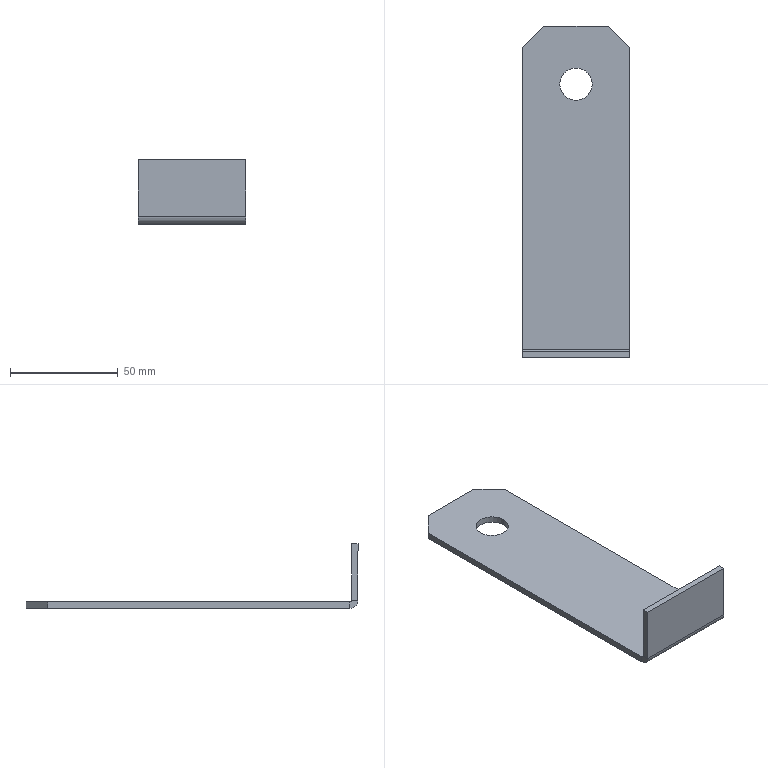Part | SolidWorks | features Chamfer 1, EdgeFlange 1, FlatPattern 1, ICE 1, SMBaseFlange 1, SheetMetal 1 | 1 solid | 18 faces | box 50 x 154 x 30 mm | volume 26176 mm3 | plane 14 | cylinder 4 | commonest cylinder face diameters 15 x2 1.473 x1 7.473 x1
STEP:
#1=CARTESIAN_POINT('',(7.5,50.,0.));
#2=VERTEX_POINT('',#1);
#3=CARTESIAN_POINT('',(-7.5,50.,0.));
#4=VERTEX_POINT('',#3);
#5=CARTESIAN_POINT('',(0.,50.,0.));
#6=DIRECTION('',(0.,0.,-1.));
#7=DIRECTION('',(-1.,0.,0.));
#8=AXIS2_PLACEMENT_3D('',#5,#6,#7);
#9=CIRCLE('',#8,7.5);
#10=EDGE_CURVE('',#2,#4,#9,.T.);
#11=ORIENTED_EDGE('',*,*,#10,.F.);
#12=CARTESIAN_POINT('',(7.5,50.,-3.));
#13=VERTEX_POINT('',#12);
#14=CARTESIAN_POINT('',(7.5,50.,27.));
#15=DIRECTION('',(0.,0.,-1.));
#16=VECTOR('',#15,1000.);
#17=LINE('',#14,#16);
#18=EDGE_CURVE('',#2,#13,#17,.T.);
#19=ORIENTED_EDGE('',*,*,#18,.T.);
#20=CARTESIAN_POINT('',(-7.5,50.,-3.));
#21=VERTEX_POINT('',#20);
#22=CARTESIAN_POINT('',(0.,50.,-3.));
#23=DIRECTION('',(0.,0.,-1.));
#24=DIRECTION('',(-1.,0.,0.));
#25=AXIS2_PLACEMENT_3D('',#22,#23,#24);
#26=CIRCLE('',#25,7.5);
#27=EDGE_CURVE('',#13,#21,#26,.T.);
#28=ORIENTED_EDGE('',*,*,#27,.T.);
#29=CARTESIAN_POINT('',(-7.5,50.,27.));
#30=DIRECTION('',(0.,0.,-1.));
#31=VECTOR('',#30,1000.);
#32=LINE('',#29,#31);
#33=EDGE_CURVE('',#4,#21,#32,.T.);
#34=ORIENTED_EDGE('',*,*,#33,.F.);
#35=EDGE_LOOP('',(#11,#19,#28,#34));
#36=FACE_OUTER_BOUND('',#35,.T.);
#37=CARTESIAN_POINT('',(0.,50.,27.));
#38=DIRECTION('',(0.,0.,-1.));
#39=DIRECTION('',(-1.,0.,0.));
#40=AXIS2_PLACEMENT_3D('',#37,#38,#39);
#41=CYLINDRICAL_SURFACE('',#40,7.5);
#42=ADVANCED_FACE('',(#36),#41,.F.);
#43=CARTESIAN_POINT('',(25.,-73.263,-3.));
#44=VERTEX_POINT('',#43);
#45=CARTESIAN_POINT('',(25.,67.,-3.));
#46=VERTEX_POINT('',#45);
#47=CARTESIAN_POINT('',(25.,-77.,-3.));
#48=DIRECTION('',(0.,1.,0.));
#49=VECTOR('',#48,1000.);
#50=LINE('',#47,#49);
#51=EDGE_CURVE('',#44,#46,#50,.T.);
#52=ORIENTED_EDGE('',*,*,#51,.T.);
#53=CARTESIAN_POINT('',(25.,67.,0.));
#54=VERTEX_POINT('',#53);
#55=CARTESIAN_POINT('',(25.,67.,-3.));
#56=DIRECTION('',(0.,0.,1.));
#57=VECTOR('',#56,1000.);
#58=LINE('',#55,#57);
#59=EDGE_CURVE('',#46,#54,#58,.T.);
#60=ORIENTED_EDGE('',*,*,#59,.T.);
#61=CARTESIAN_POINT('',(25.,-73.263,0.));
#62=VERTEX_POINT('',#61);
#63=CARTESIAN_POINT('',(25.,-77.,0.));
#64=DIRECTION('',(0.,1.,0.));
#65=VECTOR('',#64,1000.);
#66=LINE('',#63,#65);
#67=EDGE_CURVE('',#62,#54,#66,.T.);
#68=ORIENTED_EDGE('',*,*,#67,.F.);
#69=CARTESIAN_POINT('',(25.,-73.263,0.));
#70=DIRECTION('',(0.,0.,-1.));
#71=VECTOR('',#70,1000.);
#72=LINE('',#69,#71);
#73=EDGE_CURVE('',#62,#44,#72,.T.);
#74=ORIENTED_EDGE('',*,*,#73,.T.);
#75=EDGE_LOOP('',(#52,#60,#68,#74));
#76=FACE_OUTER_BOUND('',#75,.T.);
#77=CARTESIAN_POINT('',(25.,-77.,-3.));
#78=DIRECTION('',(1.,0.,0.));
#79=DIRECTION('',(0.,0.,-1.));
#80=AXIS2_PLACEMENT_3D('',#77,#78,#79);
#81=PLANE('',#80);
#82=ADVANCED_FACE('',(#76),#81,.T.);
#83=CARTESIAN_POINT('',(0.,50.,-3.));
#84=DIRECTION('',(0.,0.,-1.));
#85=DIRECTION('',(-1.,0.,0.));
#86=AXIS2_PLACEMENT_3D('',#83,#84,#85);
#87=CIRCLE('',#86,7.5);
#88=EDGE_CURVE('',#21,#13,#87,.T.);
#89=ORIENTED_EDGE('',*,*,#88,.F.);
#90=ORIENTED_EDGE('',*,*,#27,.F.);
#91=EDGE_LOOP('',(#89,#90));
#92=FACE_BOUND('',#91,.T.);
#93=CARTESIAN_POINT('',(-25.,67.,-3.));
#94=VERTEX_POINT('',#93);
#95=CARTESIAN_POINT('',(-25.,-73.263,-3.));
#96=VERTEX_POINT('',#95);
#97=CARTESIAN_POINT('',(-25.,-77.,-3.));
#98=DIRECTION('',(0.,-1.,0.));
#99=VECTOR('',#98,1000.);
#100=LINE('',#97,#99);
#101=EDGE_CURVE('',#94,#96,#100,.T.);
#102=ORIENTED_EDGE('',*,*,#101,.F.);
#103=CARTESIAN_POINT('',(-15.,77.,-3.));
#104=VERTEX_POINT('',#103);
#105=CARTESIAN_POINT('',(-46.,46.,-3.));
#106=DIRECTION('',(0.7071,0.7071,0.));
#107=VECTOR('',#106,1000.);
#108=LINE('',#105,#107);
#109=EDGE_CURVE('',#94,#104,#108,.T.);
#110=ORIENTED_EDGE('',*,*,#109,.T.);
#111=CARTESIAN_POINT('',(15.,77.,-3.));
#112=VERTEX_POINT('',#111);
#113=CARTESIAN_POINT('',(-25.,77.,-3.));
#114=DIRECTION('',(-1.,0.,0.));
#115=VECTOR('',#114,1000.);
#116=LINE('',#113,#115);
#117=EDGE_CURVE('',#112,#104,#116,.T.);
#118=ORIENTED_EDGE('',*,*,#117,.F.);
#119=CARTESIAN_POINT('',(46.,46.,-3.));
#120=DIRECTION('',(0.7071,-0.7071,0.));
#121=VECTOR('',#120,1000.);
#122=LINE('',#119,#121);
#123=EDGE_CURVE('',#112,#46,#122,.T.);
#124=ORIENTED_EDGE('',*,*,#123,.T.);
#125=ORIENTED_EDGE('',*,*,#51,.F.);
#126=CARTESIAN_POINT('',(25.,-73.263,-3.));
#127=DIRECTION('',(-1.,0.,0.));
#128=VECTOR('',#127,1000.);
#129=LINE('',#126,#128);
#130=EDGE_CURVE('',#44,#96,#129,.T.);
#131=ORIENTED_EDGE('',*,*,#130,.T.);
#132=EDGE_LOOP('',(#102,#110,#118,#124,#125,#131));
#133=FACE_OUTER_BOUND('',#132,.T.);
#134=CARTESIAN_POINT('',(0.,0.,-3.));
#135=DIRECTION('',(0.,0.,-1.));
#136=DIRECTION('',(-1.,0.,0.));
#137=AXIS2_PLACEMENT_3D('',#134,#135,#136);
#138=PLANE('',#137);
#139=ADVANCED_FACE('',(#92,#133),#138,.T.);
#140=CARTESIAN_POINT('',(0.,50.,0.));
#141=DIRECTION('',(0.,0.,-1.));
#142=DIRECTION('',(-1.,0.,0.));
#143=AXIS2_PLACEMENT_3D('',#140,#141,#142);
#144=CIRCLE('',#143,7.5);
#145=EDGE_CURVE('',#4,#2,#144,.T.);
#146=ORIENTED_EDGE('',*,*,#145,.T.);
#147=ORIENTED_EDGE('',*,*,#10,.T.);
#148=EDGE_LOOP('',(#146,#147));
#149=FACE_BOUND('',#148,.T.);
#150=CARTESIAN_POINT('',(15.,77.,0.));
#151=VERTEX_POINT('',#150);
#152=CARTESIAN_POINT('',(-15.,77.,0.));
#153=VERTEX_POINT('',#152);
#154=CARTESIAN_POINT('',(-25.,77.,0.));
#155=DIRECTION('',(-1.,0.,0.));
#156=VECTOR('',#155,1000.);
#157=LINE('',#154,#156);
#158=EDGE_CURVE('',#151,#153,#157,.T.);
#159=ORIENTED_EDGE('',*,*,#158,.T.);
#160=CARTESIAN_POINT('',(-25.,67.,0.));
#161=VERTEX_POINT('',#160);
#162=CARTESIAN_POINT('',(-15.,77.,0.));
#163=DIRECTION('',(-0.7071,-0.7071,0.));
#164=VECTOR('',#163,1000.);
#165=LINE('',#162,#164);
#166=EDGE_CURVE('',#153,#161,#165,.T.);
#167=ORIENTED_EDGE('',*,*,#166,.T.);
#168=CARTESIAN_POINT('',(-25.,-73.263,0.));
#169=VERTEX_POINT('',#168);
#170=CARTESIAN_POINT('',(-25.,-77.,0.));
#171=DIRECTION('',(0.,-1.,0.));
#172=VECTOR('',#171,1000.);
#173=LINE('',#170,#172);
#174=EDGE_CURVE('',#161,#169,#173,.T.);
#175=ORIENTED_EDGE('',*,*,#174,.T.);
#176=CARTESIAN_POINT('',(25.,-73.263,0.));
#177=DIRECTION('',(-1.,0.,0.));
#178=VECTOR('',#177,1000.);
#179=LINE('',#176,#178);
#180=EDGE_CURVE('',#62,#169,#179,.T.);
#181=ORIENTED_EDGE('',*,*,#180,.F.);
#182=ORIENTED_EDGE('',*,*,#67,.T.);
#183=CARTESIAN_POINT('',(25.,67.,0.));
#184=DIRECTION('',(-0.7071,0.7071,0.));
#185=VECTOR('',#184,1000.);
#186=LINE('',#183,#185);
#187=EDGE_CURVE('',#54,#151,#186,.T.);
#188=ORIENTED_EDGE('',*,*,#187,.T.);
#189=EDGE_LOOP('',(#159,#167,#175,#181,#182,#188));
#190=FACE_OUTER_BOUND('',#189,.T.);
#191=CARTESIAN_POINT('',(0.,0.,0.));
#192=DIRECTION('',(0.,0.,-1.));
#193=DIRECTION('',(-1.,0.,0.));
#194=AXIS2_PLACEMENT_3D('',#191,#192,#193);
#195=PLANE('',#194);
#196=ADVANCED_FACE('',(#149,#190),#195,.F.);
#197=ORIENTED_EDGE('',*,*,#174,.F.);
#198=CARTESIAN_POINT('',(-25.,67.,-3.));
#199=DIRECTION('',(0.,0.,-1.));
#200=VECTOR('',#199,1000.);
#201=LINE('',#198,#200);
#202=EDGE_CURVE('',#161,#94,#201,.T.);
#203=ORIENTED_EDGE('',*,*,#202,.T.);
#204=ORIENTED_EDGE('',*,*,#101,.T.);
#205=CARTESIAN_POINT('',(-25.,-73.263,0.));
#206=DIRECTION('',(0.,0.,-1.));
#207=VECTOR('',#206,1000.);
#208=LINE('',#205,#207);
#209=EDGE_CURVE('',#169,#96,#208,.T.);
#210=ORIENTED_EDGE('',*,*,#209,.F.);
#211=EDGE_LOOP('',(#197,#203,#204,#210));
#212=FACE_OUTER_BOUND('',#211,.T.);
#213=CARTESIAN_POINT('',(-25.,-77.,-3.));
#214=DIRECTION('',(-1.,0.,0.));
#215=DIRECTION('',(0.,0.,1.));
#216=AXIS2_PLACEMENT_3D('',#213,#214,#215);
#217=PLANE('',#216);
#218=ADVANCED_FACE('',(#212),#217,.T.);
#219=ORIENTED_EDGE('',*,*,#117,.T.);
#220=CARTESIAN_POINT('',(-15.,77.,-3.));
#221=DIRECTION('',(0.,0.,1.));
#222=VECTOR('',#221,1000.);
#223=LINE('',#220,#222);
#224=EDGE_CURVE('',#104,#153,#223,.T.);
#225=ORIENTED_EDGE('',*,*,#224,.T.);
#226=ORIENTED_EDGE('',*,*,#158,.F.);
#227=CARTESIAN_POINT('',(15.,77.,-3.));
#228=DIRECTION('',(0.,0.,-1.));
#229=VECTOR('',#228,1000.);
#230=LINE('',#227,#229);
#231=EDGE_CURVE('',#151,#112,#230,.T.);
#232=ORIENTED_EDGE('',*,*,#231,.T.);
#233=EDGE_LOOP('',(#219,#225,#226,#232));
#234=FACE_OUTER_BOUND('',#233,.T.);
#235=CARTESIAN_POINT('',(-25.,77.,-3.));
#236=DIRECTION('',(0.,1.,0.));
#237=DIRECTION('',(0.,0.,1.));
#238=AXIS2_PLACEMENT_3D('',#235,#236,#237);
#239=PLANE('',#238);
#240=ADVANCED_FACE('',(#234),#239,.T.);
#241=CARTESIAN_POINT('',(-25.,-74.,0.7366));
#242=VERTEX_POINT('',#241);
#243=CARTESIAN_POINT('',(-25.,-77.,0.7366));
#244=VERTEX_POINT('',#243);
#245=CARTESIAN_POINT('',(-25.,-77.,0.7366));
#246=DIRECTION('',(0.,-1.,0.));
#247=VECTOR('',#246,1000.);
#248=LINE('',#245,#247);
#249=EDGE_CURVE('',#242,#244,#248,.T.);
#250=ORIENTED_EDGE('',*,*,#249,.F.);
#251=CARTESIAN_POINT('',(-25.,-73.263,0.7366));
#252=DIRECTION('',(-1.,0.,0.));
#253=DIRECTION('',(0.,0.,-1.));
#254=AXIS2_PLACEMENT_3D('',#251,#252,#253);
#255=CIRCLE('',#254,0.7366);
#256=EDGE_CURVE('',#169,#242,#255,.T.);
#257=ORIENTED_EDGE('',*,*,#256,.F.);
#258=ORIENTED_EDGE('',*,*,#209,.T.);
#259=CARTESIAN_POINT('',(-25.,-73.263,0.7366));
#260=DIRECTION('',(-1.,0.,0.));
#261=DIRECTION('',(0.,0.,-1.));
#262=AXIS2_PLACEMENT_3D('',#259,#260,#261);
#263=CIRCLE('',#262,3.737);
#264=EDGE_CURVE('',#96,#244,#263,.T.);
#265=ORIENTED_EDGE('',*,*,#264,.T.);
#266=EDGE_LOOP('',(#250,#257,#258,#265));
#267=FACE_OUTER_BOUND('',#266,.T.);
#268=CARTESIAN_POINT('',(-25.,-73.263,0.7366));
#269=DIRECTION('',(-1.,0.,0.));
#270=DIRECTION('',(0.,0.,1.));
#271=AXIS2_PLACEMENT_3D('',#268,#269,#270);
#272=PLANE('',#271);
#273=ADVANCED_FACE('',(#267),#272,.T.);
#274=CARTESIAN_POINT('',(25.,-74.,0.7366));
#275=VERTEX_POINT('',#274);
#276=CARTESIAN_POINT('',(25.,-73.263,0.7366));
#277=DIRECTION('',(1.,0.,0.));
#278=DIRECTION('',(0.,0.,-1.));
#279=AXIS2_PLACEMENT_3D('',#276,#277,#278);
#280=CIRCLE('',#279,0.7366);
#281=EDGE_CURVE('',#275,#62,#280,.T.);
#282=ORIENTED_EDGE('',*,*,#281,.F.);
#283=CARTESIAN_POINT('',(25.,-77.,0.7366));
#284=VERTEX_POINT('',#283);
#285=CARTESIAN_POINT('',(25.,-74.,0.7366));
#286=DIRECTION('',(0.,-1.,0.));
#287=VECTOR('',#286,1000.);
#288=LINE('',#285,#287);
#289=EDGE_CURVE('',#275,#284,#288,.T.);
#290=ORIENTED_EDGE('',*,*,#289,.T.);
#291=CARTESIAN_POINT('',(25.,-73.263,0.7366));
#292=DIRECTION('',(1.,0.,0.));
#293=DIRECTION('',(0.,0.,-1.));
#294=AXIS2_PLACEMENT_3D('',#291,#292,#293);
#295=CIRCLE('',#294,3.737);
#296=EDGE_CURVE('',#284,#44,#295,.T.);
#297=ORIENTED_EDGE('',*,*,#296,.T.);
#298=ORIENTED_EDGE('',*,*,#73,.F.);
#299=EDGE_LOOP('',(#282,#290,#297,#298));
#300=FACE_OUTER_BOUND('',#299,.T.);
#301=CARTESIAN_POINT('',(25.,-73.263,0.7366));
#302=DIRECTION('',(-1.,0.,0.));
#303=DIRECTION('',(0.,0.,1.));
#304=AXIS2_PLACEMENT_3D('',#301,#302,#303);
#305=PLANE('',#304);
#306=ADVANCED_FACE('',(#300),#305,.F.);
#307=ORIENTED_EDGE('',*,*,#130,.F.);
#308=ORIENTED_EDGE('',*,*,#296,.F.);
#309=CARTESIAN_POINT('',(-25.,-77.,0.7366));
#310=DIRECTION('',(-1.,0.,0.));
#311=VECTOR('',#310,1000.);
#312=LINE('',#309,#311);
#313=EDGE_CURVE('',#284,#244,#312,.T.);
#314=ORIENTED_EDGE('',*,*,#313,.T.);
#315=ORIENTED_EDGE('',*,*,#264,.F.);
#316=EDGE_LOOP('',(#307,#308,#314,#315));
#317=FACE_OUTER_BOUND('',#316,.T.);
#318=CARTESIAN_POINT('',(25.,-73.263,0.7366));
#319=DIRECTION('',(1.,0.,0.));
#320=DIRECTION('',(0.,-1.,0.));
#321=AXIS2_PLACEMENT_3D('',#318,#319,#320);
#322=CYLINDRICAL_SURFACE('',#321,3.737);
#323=ADVANCED_FACE('',(#317),#322,.T.);
#324=ORIENTED_EDGE('',*,*,#180,.T.);
#325=ORIENTED_EDGE('',*,*,#256,.T.);
#326=CARTESIAN_POINT('',(-25.,-74.,0.7366));
#327=DIRECTION('',(1.,0.,0.));
#328=VECTOR('',#327,1000.);
#329=LINE('',#326,#328);
#330=EDGE_CURVE('',#242,#275,#329,.T.);
#331=ORIENTED_EDGE('',*,*,#330,.T.);
#332=ORIENTED_EDGE('',*,*,#281,.T.);
#333=EDGE_LOOP('',(#324,#325,#331,#332));
#334=FACE_OUTER_BOUND('',#333,.T.);
#335=CARTESIAN_POINT('',(25.,-73.263,0.7366));
#336=DIRECTION('',(1.,0.,0.));
#337=DIRECTION('',(0.,-1.,0.));
#338=AXIS2_PLACEMENT_3D('',#335,#336,#337);
#339=CYLINDRICAL_SURFACE('',#338,0.7366);
#340=ADVANCED_FACE('',(#334),#339,.F.);
#341=ORIENTED_EDGE('',*,*,#249,.T.);
#342=CARTESIAN_POINT('',(-25.,-77.,27.));
#343=VERTEX_POINT('',#342);
#344=CARTESIAN_POINT('',(-25.,-77.,0.));
#345=DIRECTION('',(0.,0.,-1.));
#346=VECTOR('',#345,1000.);
#347=LINE('',#344,#346);
#348=EDGE_CURVE('',#343,#244,#347,.T.);
#349=ORIENTED_EDGE('',*,*,#348,.F.);
#350=CARTESIAN_POINT('',(-25.,-74.,27.));
#351=VERTEX_POINT('',#350);
#352=CARTESIAN_POINT('',(-25.,-77.,27.));
#353=DIRECTION('',(0.,1.,0.));
#354=VECTOR('',#353,1000.);
#355=LINE('',#352,#354);
#356=EDGE_CURVE('',#343,#351,#355,.T.);
#357=ORIENTED_EDGE('',*,*,#356,.T.);
#358=CARTESIAN_POINT('',(-25.,-74.,0.));
#359=DIRECTION('',(0.,0.,-1.));
#360=VECTOR('',#359,1000.);
#361=LINE('',#358,#360);
#362=EDGE_CURVE('',#351,#242,#361,.T.);
#363=ORIENTED_EDGE('',*,*,#362,.T.);
#364=EDGE_LOOP('',(#341,#349,#357,#363));
#365=FACE_OUTER_BOUND('',#364,.T.);
#366=CARTESIAN_POINT('',(-25.,-77.,0.));
#367=DIRECTION('',(1.,0.,0.));
#368=DIRECTION('',(0.,0.,-1.));
#369=AXIS2_PLACEMENT_3D('',#366,#367,#368);
#370=PLANE('',#369);
#371=ADVANCED_FACE('',(#365),#370,.F.);
#372=ORIENTED_EDGE('',*,*,#289,.F.);
#373=CARTESIAN_POINT('',(25.,-74.,27.));
#374=VERTEX_POINT('',#373);
#375=CARTESIAN_POINT('',(25.,-74.,27.));
#376=DIRECTION('',(0.,0.,1.));
#377=VECTOR('',#376,1000.);
#378=LINE('',#375,#377);
#379=EDGE_CURVE('',#275,#374,#378,.T.);
#380=ORIENTED_EDGE('',*,*,#379,.T.);
#381=CARTESIAN_POINT('',(25.,-77.,27.));
#382=VERTEX_POINT('',#381);
#383=CARTESIAN_POINT('',(25.,-77.,27.));
#384=DIRECTION('',(0.,1.,0.));
#385=VECTOR('',#384,1000.);
#386=LINE('',#383,#385);
#387=EDGE_CURVE('',#382,#374,#386,.T.);
#388=ORIENTED_EDGE('',*,*,#387,.F.);
#389=CARTESIAN_POINT('',(25.,-77.,0.));
#390=DIRECTION('',(0.,0.,1.));
#391=VECTOR('',#390,1000.);
#392=LINE('',#389,#391);
#393=EDGE_CURVE('',#284,#382,#392,.T.);
#394=ORIENTED_EDGE('',*,*,#393,.F.);
#395=EDGE_LOOP('',(#372,#380,#388,#394));
#396=FACE_OUTER_BOUND('',#395,.T.);
#397=CARTESIAN_POINT('',(25.,-77.,27.));
#398=DIRECTION('',(-1.,0.,0.));
#399=DIRECTION('',(0.,0.,1.));
#400=AXIS2_PLACEMENT_3D('',#397,#398,#399);
#401=PLANE('',#400);
#402=ADVANCED_FACE('',(#396),#401,.F.);
#403=ORIENTED_EDGE('',*,*,#313,.F.);
#404=ORIENTED_EDGE('',*,*,#393,.T.);
#405=CARTESIAN_POINT('',(0.,-77.,27.));
#406=DIRECTION('',(-1.,0.,0.));
#407=VECTOR('',#406,1000.);
#408=LINE('',#405,#407);
#409=EDGE_CURVE('',#382,#343,#408,.T.);
#410=ORIENTED_EDGE('',*,*,#409,.T.);
#411=ORIENTED_EDGE('',*,*,#348,.T.);
#412=EDGE_LOOP('',(#403,#404,#410,#411));
#413=FACE_OUTER_BOUND('',#412,.T.);
#414=CARTESIAN_POINT('',(0.,-77.,0.));
#415=DIRECTION('',(0.,1.,0.));
#416=DIRECTION('',(0.,0.,1.));
#417=AXIS2_PLACEMENT_3D('',#414,#415,#416);
#418=PLANE('',#417);
#419=ADVANCED_FACE('',(#413),#418,.F.);
#420=ORIENTED_EDGE('',*,*,#379,.F.);
#421=ORIENTED_EDGE('',*,*,#330,.F.);
#422=ORIENTED_EDGE('',*,*,#362,.F.);
#423=CARTESIAN_POINT('',(-25.,-74.,27.));
#424=DIRECTION('',(-1.,0.,0.));
#425=VECTOR('',#424,1000.);
#426=LINE('',#423,#425);
#427=EDGE_CURVE('',#374,#351,#426,.T.);
#428=ORIENTED_EDGE('',*,*,#427,.F.);
#429=EDGE_LOOP('',(#420,#421,#422,#428));
#430=FACE_OUTER_BOUND('',#429,.T.);
#431=CARTESIAN_POINT('',(0.,-74.,0.));
#432=DIRECTION('',(0.,1.,0.));
#433=DIRECTION('',(0.,0.,1.));
#434=AXIS2_PLACEMENT_3D('',#431,#432,#433);
#435=PLANE('',#434);
#436=ADVANCED_FACE('',(#430),#435,.T.);
#437=ORIENTED_EDGE('',*,*,#427,.T.);
#438=ORIENTED_EDGE('',*,*,#356,.F.);
#439=ORIENTED_EDGE('',*,*,#409,.F.);
#440=ORIENTED_EDGE('',*,*,#387,.T.);
#441=EDGE_LOOP('',(#437,#438,#439,#440));
#442=FACE_OUTER_BOUND('',#441,.T.);
#443=CARTESIAN_POINT('',(-25.,-77.,27.));
#444=DIRECTION('',(0.,0.,-1.));
#445=DIRECTION('',(0.,1.,0.));
#446=AXIS2_PLACEMENT_3D('',#443,#444,#445);
#447=PLANE('',#446);
#448=ADVANCED_FACE('',(#442),#447,.F.);
#449=ORIENTED_EDGE('',*,*,#18,.F.);
#450=ORIENTED_EDGE('',*,*,#145,.F.);
#451=ORIENTED_EDGE('',*,*,#33,.T.);
#452=ORIENTED_EDGE('',*,*,#88,.T.);
#453=EDGE_LOOP('',(#449,#450,#451,#452));
#454=FACE_OUTER_BOUND('',#453,.T.);
#455=CARTESIAN_POINT('',(0.,50.,27.));
#456=DIRECTION('',(0.,0.,-1.));
#457=DIRECTION('',(-1.,0.,0.));
#458=AXIS2_PLACEMENT_3D('',#455,#456,#457);
#459=CYLINDRICAL_SURFACE('',#458,7.5);
#460=ADVANCED_FACE('',(#454),#459,.F.);
#461=ORIENTED_EDGE('',*,*,#109,.F.);
#462=ORIENTED_EDGE('',*,*,#202,.F.);
#463=ORIENTED_EDGE('',*,*,#166,.F.);
#464=ORIENTED_EDGE('',*,*,#224,.F.);
#465=EDGE_LOOP('',(#461,#462,#463,#464));
#466=FACE_OUTER_BOUND('',#465,.T.);
#467=CARTESIAN_POINT('',(-15.,77.,-3.));
#468=DIRECTION('',(0.7071,-0.7071,0.));
#469=DIRECTION('',(0.,0.,1.));
#470=AXIS2_PLACEMENT_3D('',#467,#468,#469);
#471=PLANE('',#470);
#472=ADVANCED_FACE('',(#466),#471,.F.);
#473=ORIENTED_EDGE('',*,*,#123,.F.);
#474=ORIENTED_EDGE('',*,*,#231,.F.);
#475=ORIENTED_EDGE('',*,*,#187,.F.);
#476=ORIENTED_EDGE('',*,*,#59,.F.);
#477=EDGE_LOOP('',(#473,#474,#475,#476));
#478=FACE_OUTER_BOUND('',#477,.T.);
#479=CARTESIAN_POINT('',(25.,67.,-3.));
#480=DIRECTION('',(-0.7071,-0.7071,0.));
#481=DIRECTION('',(0.,0.,1.));
#482=AXIS2_PLACEMENT_3D('',#479,#480,#481);
#483=PLANE('',#482);
#484=ADVANCED_FACE('',(#478),#483,.F.);
#485=CLOSED_SHELL('',(#42,#82,#139,#196,#218,#240,#273,#306,#323,#340,#371,#402,#419,#436,#448,#460,#472,#484));
#486=MANIFOLD_SOLID_BREP('',#485);
#487=CARTESIAN_POINT('',(0.,0.,0.));
#488=DIRECTION('',(0.,0.,1.));
#489=DIRECTION('',(1.,0.,0.));
#490=AXIS2_PLACEMENT_3D('',#487,#488,#489);
#491=(LENGTH_UNIT()NAMED_UNIT(*)SI_UNIT(.MILLI.,.METRE.));
#492=UNCERTAINTY_MEASURE_WITH_UNIT(LENGTH_MEASURE(0.00001),#491,'','');
#493=(NAMED_UNIT(*)PLANE_ANGLE_UNIT()SI_UNIT($,.RADIAN.));
#494=(NAMED_UNIT(*)SI_UNIT($,.STERADIAN.)SOLID_ANGLE_UNIT());
#495=(GEOMETRIC_REPRESENTATION_CONTEXT(3)GLOBAL_UNCERTAINTY_ASSIGNED_CONTEXT((#492))GLOBAL_UNIT_ASSIGNED_CONTEXT((#491,#493,#494))REPRESENTATION_CONTEXT('',''));
#496=ADVANCED_BREP_SHAPE_REPRESENTATION('',(#486,#490),#495);